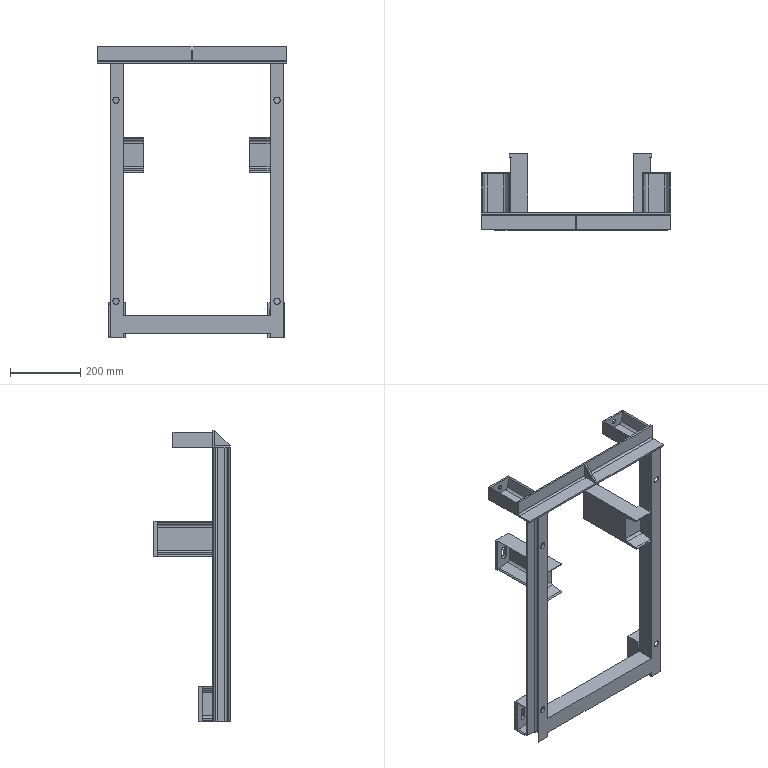Part | SolidWorks | features BaseBody 5 | 5 solids | 182 faces | box 540 x 218 x 834 mm | volume 2399643 mm3 | plane 113 | cylinder 69 | commonest cylinder face diameters 8 x16 16 x16 14 x14 18 x14 7 x4 4 x2